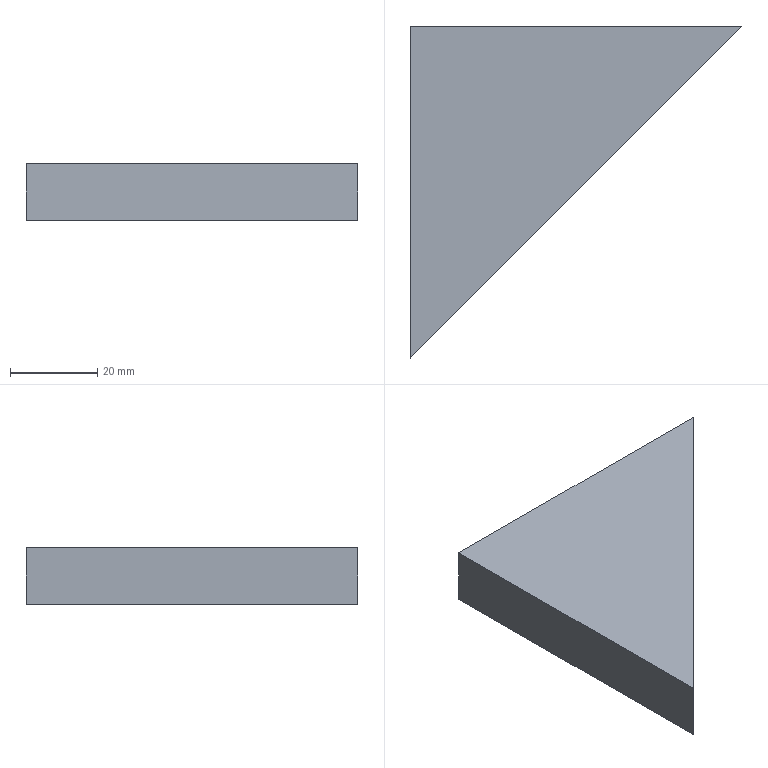Part | SolidWorks | features BaseBody 1 | 1 solid | 5 faces | box 76 x 76 x 13 mm | volume 37544 mm3 | plane 5
STEP:
#1=CARTESIAN_POINT('',(-5.397,-1.313,0.));
#2=VERTEX_POINT('',#1);
#3=CARTESIAN_POINT('',(70.603,74.687,0.));
#4=VERTEX_POINT('',#3);
#5=CARTESIAN_POINT('',(-5.397,-1.313,0.));
#6=DIRECTION('',(0.7071,0.7071,0.));
#7=VECTOR('',#6,1000.);
#8=LINE('',#5,#7);
#9=EDGE_CURVE('',#2,#4,#8,.T.);
#10=ORIENTED_EDGE('',*,*,#9,.F.);
#11=CARTESIAN_POINT('',(-5.397,74.687,0.));
#12=VERTEX_POINT('',#11);
#13=CARTESIAN_POINT('',(-5.397,47.817,0.));
#14=DIRECTION('',(0.,-1.,0.));
#15=VECTOR('',#14,1000.);
#16=LINE('',#13,#15);
#17=EDGE_CURVE('',#12,#2,#16,.T.);
#18=ORIENTED_EDGE('',*,*,#17,.F.);
#19=CARTESIAN_POINT('',(21.473,74.687,0.));
#20=DIRECTION('',(-1.,0.,0.));
#21=VECTOR('',#20,1000.);
#22=LINE('',#19,#21);
#23=EDGE_CURVE('',#4,#12,#22,.T.);
#24=ORIENTED_EDGE('',*,*,#23,.F.);
#25=EDGE_LOOP('',(#10,#18,#24));
#26=FACE_OUTER_BOUND('',#25,.T.);
#27=CARTESIAN_POINT('',(21.473,47.817,0.));
#28=DIRECTION('',(0.,0.,1.));
#29=DIRECTION('',(1.,0.,0.));
#30=AXIS2_PLACEMENT_3D('',#27,#28,#29);
#31=PLANE('',#30);
#32=ADVANCED_FACE('',(#26),#31,.F.);
#33=ORIENTED_EDGE('',*,*,#23,.T.);
#34=CARTESIAN_POINT('',(-5.397,74.687,13.));
#35=VERTEX_POINT('',#34);
#36=CARTESIAN_POINT('',(-5.397,74.687,0.));
#37=DIRECTION('',(0.,0.,1.));
#38=VECTOR('',#37,1000.);
#39=LINE('',#36,#38);
#40=EDGE_CURVE('',#12,#35,#39,.T.);
#41=ORIENTED_EDGE('',*,*,#40,.T.);
#42=CARTESIAN_POINT('',(70.603,74.687,13.));
#43=VERTEX_POINT('',#42);
#44=CARTESIAN_POINT('',(-5.397,74.687,13.));
#45=DIRECTION('',(1.,0.,0.));
#46=VECTOR('',#45,1000.);
#47=LINE('',#44,#46);
#48=EDGE_CURVE('',#35,#43,#47,.T.);
#49=ORIENTED_EDGE('',*,*,#48,.T.);
#50=CARTESIAN_POINT('',(70.603,74.687,0.));
#51=DIRECTION('',(0.,0.,-1.));
#52=VECTOR('',#51,1000.);
#53=LINE('',#50,#52);
#54=EDGE_CURVE('',#43,#4,#53,.T.);
#55=ORIENTED_EDGE('',*,*,#54,.T.);
#56=EDGE_LOOP('',(#33,#41,#49,#55));
#57=FACE_OUTER_BOUND('',#56,.T.);
#58=CARTESIAN_POINT('',(-5.397,74.687,0.));
#59=DIRECTION('',(0.,1.,0.));
#60=DIRECTION('',(0.,0.,1.));
#61=AXIS2_PLACEMENT_3D('',#58,#59,#60);
#62=PLANE('',#61);
#63=ADVANCED_FACE('',(#57),#62,.T.);
#64=ORIENTED_EDGE('',*,*,#9,.T.);
#65=ORIENTED_EDGE('',*,*,#54,.F.);
#66=CARTESIAN_POINT('',(-5.397,-1.313,13.));
#67=VERTEX_POINT('',#66);
#68=CARTESIAN_POINT('',(70.603,74.687,13.));
#69=DIRECTION('',(-0.7071,-0.7071,0.));
#70=VECTOR('',#69,1000.);
#71=LINE('',#68,#70);
#72=EDGE_CURVE('',#43,#67,#71,.T.);
#73=ORIENTED_EDGE('',*,*,#72,.T.);
#74=CARTESIAN_POINT('',(-5.397,-1.313,0.));
#75=DIRECTION('',(0.,0.,-1.));
#76=VECTOR('',#75,1000.);
#77=LINE('',#74,#76);
#78=EDGE_CURVE('',#67,#2,#77,.T.);
#79=ORIENTED_EDGE('',*,*,#78,.T.);
#80=EDGE_LOOP('',(#64,#65,#73,#79));
#81=FACE_OUTER_BOUND('',#80,.T.);
#82=CARTESIAN_POINT('',(70.603,74.687,0.));
#83=DIRECTION('',(0.7071,-0.7071,0.));
#84=DIRECTION('',(0.7071,0.7071,0.));
#85=AXIS2_PLACEMENT_3D('',#82,#83,#84);
#86=PLANE('',#85);
#87=ADVANCED_FACE('',(#81),#86,.T.);
#88=ORIENTED_EDGE('',*,*,#17,.T.);
#89=ORIENTED_EDGE('',*,*,#78,.F.);
#90=CARTESIAN_POINT('',(-5.397,-1.313,13.));
#91=DIRECTION('',(0.,1.,0.));
#92=VECTOR('',#91,1000.);
#93=LINE('',#90,#92);
#94=EDGE_CURVE('',#67,#35,#93,.T.);
#95=ORIENTED_EDGE('',*,*,#94,.T.);
#96=ORIENTED_EDGE('',*,*,#40,.F.);
#97=EDGE_LOOP('',(#88,#89,#95,#96));
#98=FACE_OUTER_BOUND('',#97,.T.);
#99=CARTESIAN_POINT('',(-5.397,-1.313,0.));
#100=DIRECTION('',(-1.,0.,0.));
#101=DIRECTION('',(0.,0.,1.));
#102=AXIS2_PLACEMENT_3D('',#99,#100,#101);
#103=PLANE('',#102);
#104=ADVANCED_FACE('',(#98),#103,.T.);
#105=ORIENTED_EDGE('',*,*,#48,.F.);
#106=ORIENTED_EDGE('',*,*,#94,.F.);
#107=ORIENTED_EDGE('',*,*,#72,.F.);
#108=EDGE_LOOP('',(#105,#106,#107));
#109=FACE_OUTER_BOUND('',#108,.T.);
#110=CARTESIAN_POINT('',(21.473,47.817,13.));
#111=DIRECTION('',(0.,0.,1.));
#112=DIRECTION('',(1.,0.,0.));
#113=AXIS2_PLACEMENT_3D('',#110,#111,#112);
#114=PLANE('',#113);
#115=ADVANCED_FACE('',(#109),#114,.T.);
#116=CLOSED_SHELL('',(#32,#63,#87,#104,#115));
#117=MANIFOLD_SOLID_BREP('',#116);
#118=CARTESIAN_POINT('',(0.,0.,0.));
#119=DIRECTION('',(0.,0.,1.));
#120=DIRECTION('',(1.,0.,0.));
#121=AXIS2_PLACEMENT_3D('',#118,#119,#120);
#122=(LENGTH_UNIT()NAMED_UNIT(*)SI_UNIT(.MILLI.,.METRE.));
#123=UNCERTAINTY_MEASURE_WITH_UNIT(LENGTH_MEASURE(0.00001),#122,'','');
#124=(NAMED_UNIT(*)PLANE_ANGLE_UNIT()SI_UNIT($,.RADIAN.));
#125=(NAMED_UNIT(*)SI_UNIT($,.STERADIAN.)SOLID_ANGLE_UNIT());
#126=(GEOMETRIC_REPRESENTATION_CONTEXT(3)GLOBAL_UNCERTAINTY_ASSIGNED_CONTEXT((#123))GLOBAL_UNIT_ASSIGNED_CONTEXT((#122,#124,#125))REPRESENTATION_CONTEXT('',''));
#127=ADVANCED_BREP_SHAPE_REPRESENTATION('',(#117,#121),#126);